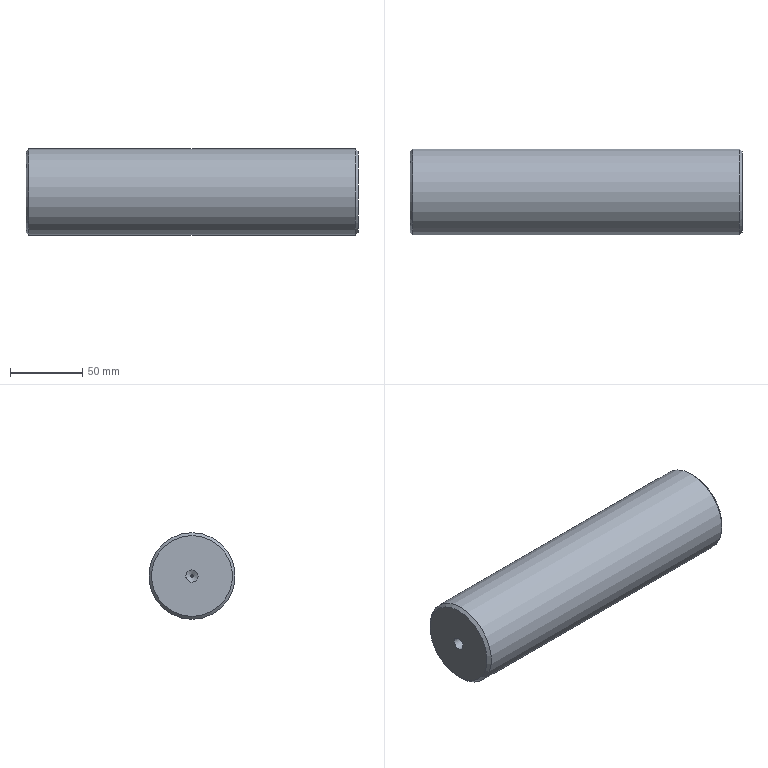Part | STEP file | solid 14 | 1 solid | 8 faces | box 230 x 60 x 60 mm | volume 648335 mm3 | plane 3 | cone 3 | cylinder 2 | commonest cylinder face diameters 8.5 x1 60 x1